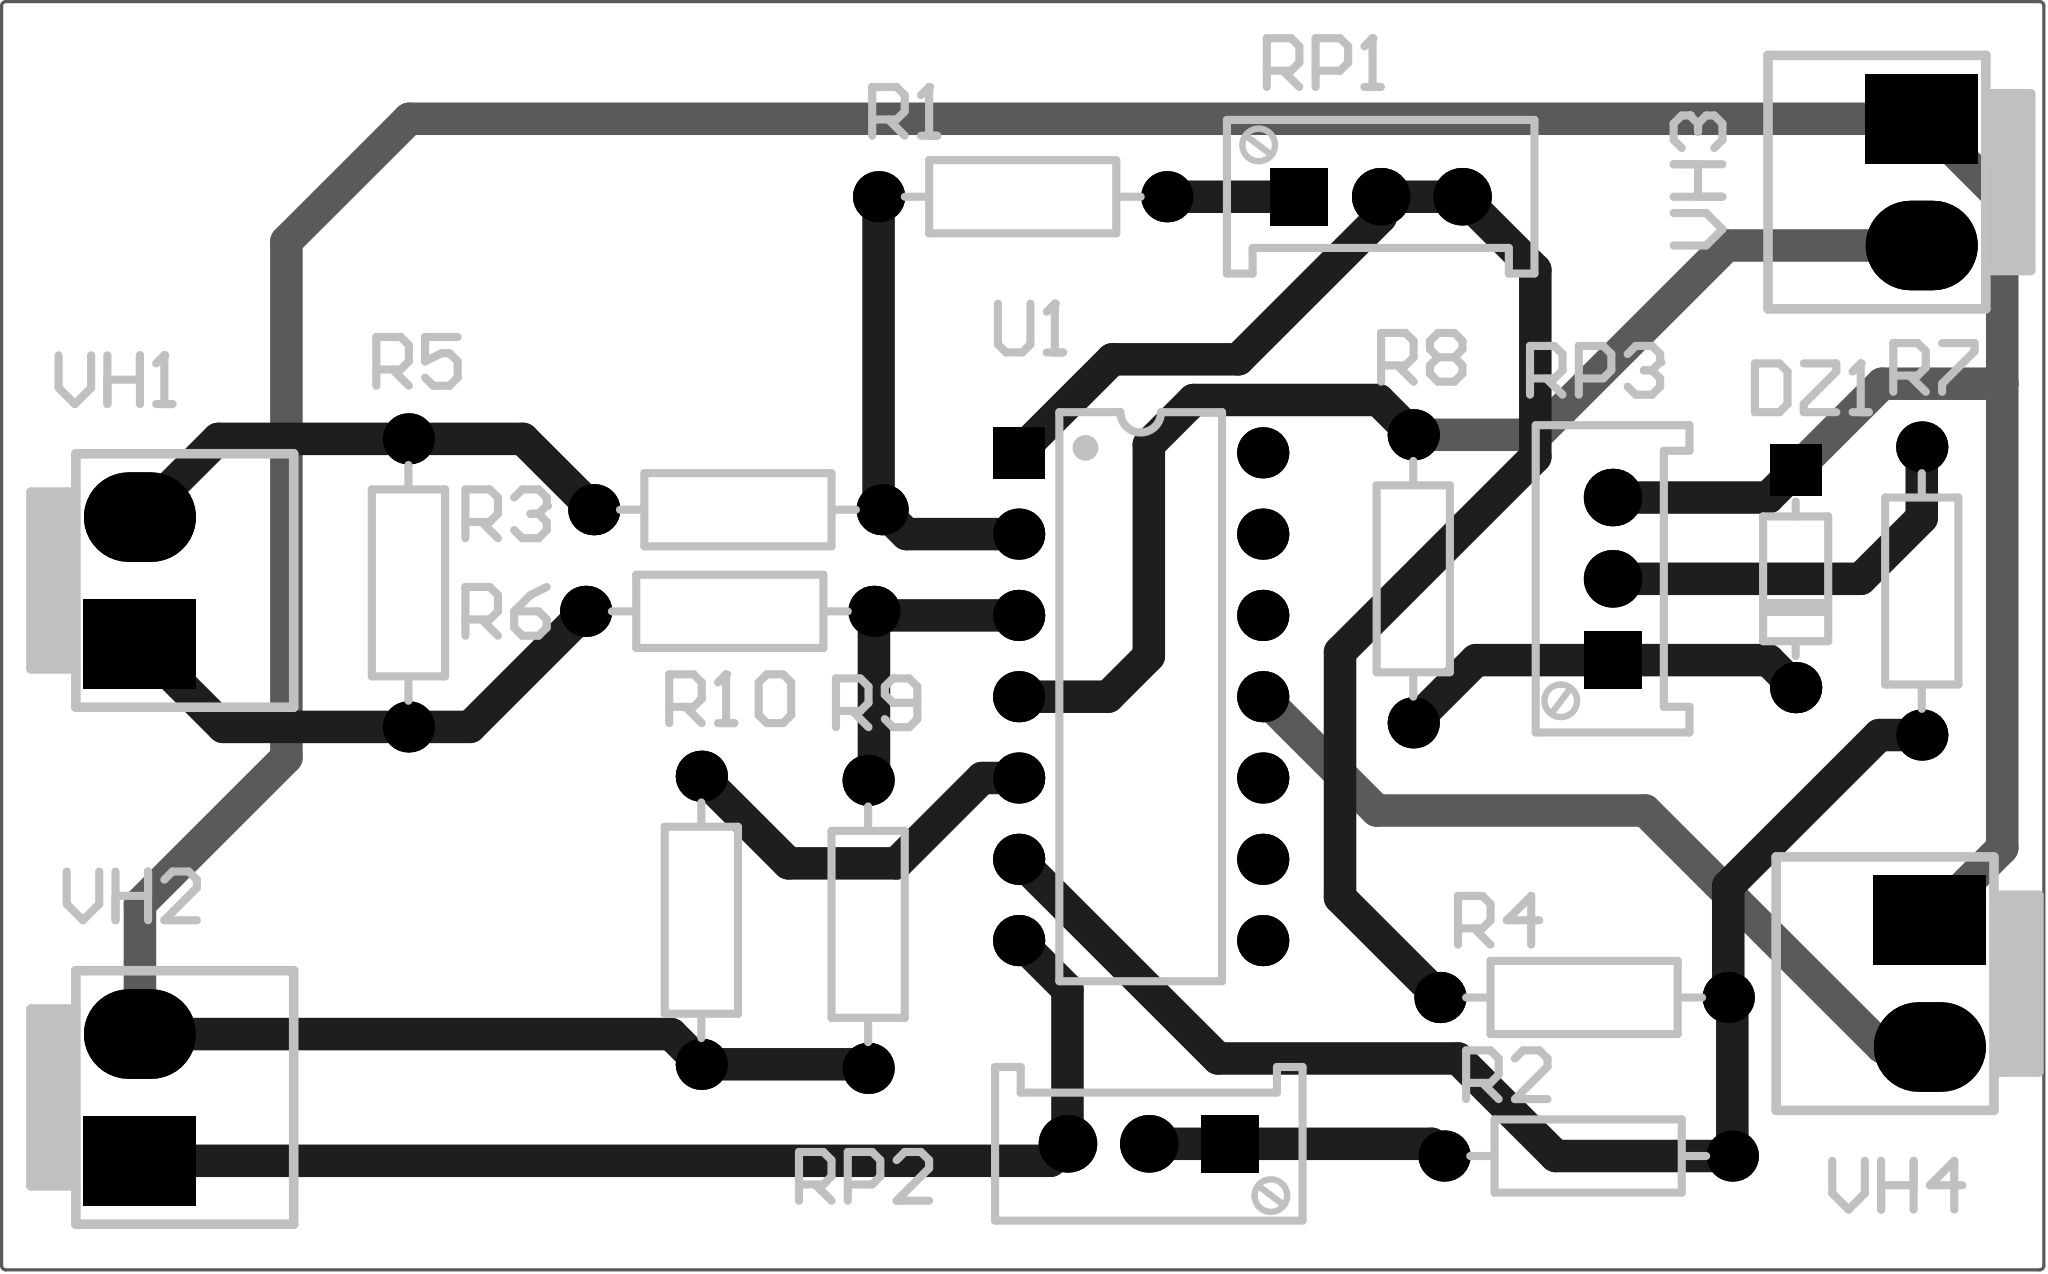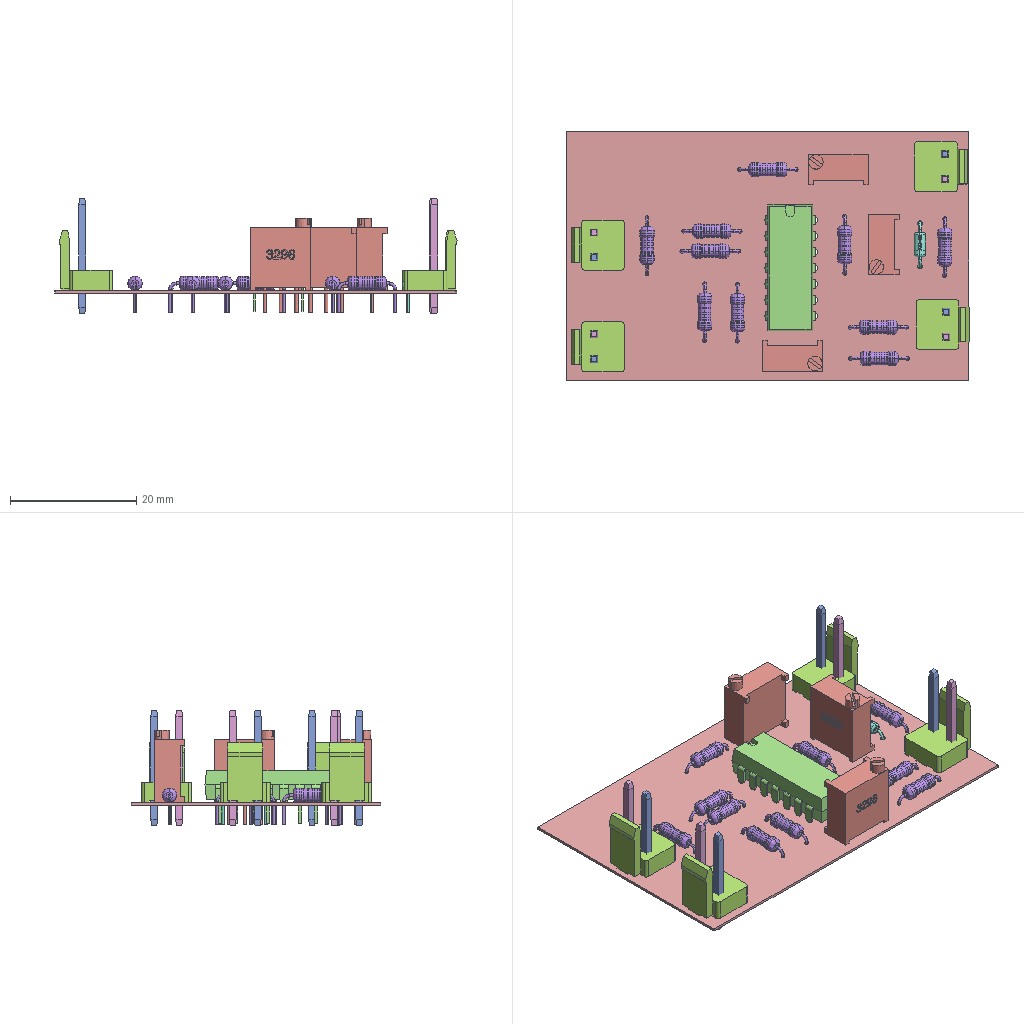Circuit board layout | Altium Designer | box 63.8 x 39.6 x 18.2 mm
Layer stack:
# Altium Designer layer stack of  (unit mm; dielectric type: 0 none, 1 core, 2 prepreg, 3 surface material)
index,name,kind,layer,copper_thickness_mm,dielectric_type,dielectric_thickness_mm,dielectric_material,dielectric_constant
0,Top Paste,other,,,,,,
1,Top Overlay,other,,,,,,
2,Top Solder,dielectric,,,3,0.0102,Solder Resist,3.5
3,Top Layer,copper,Top Layer,0.0356,,,,
4,Dielectric 1,dielectric,,,0,0.32,FR-4,4.8
5,Bottom Layer,copper,Bottom Layer,0.0356,,,,
6,Bottom Solder,dielectric,,,3,0.0102,Solder Resist,3.5
7,Bottom Overlay,other,,,,,,
8,Bottom Paste,other,,,,,,
# drill layer pairs: low layer,high layer
drill_pair,Top Layer,Bottom Layer
Part placement:
Designator,Comment,Layer,Footprint,Center-X(mm),Center-Y(mm),Rotation
VH4,VH2,TopLayer,VH3.96-2A,122.301,34.215,270
VH3,VH2,TopLayer,VH3.96-2A,122.047,59.257,270
DZ1,6V2,TopLayer,DO-35,118.11,46.863,270
R1,9.1K,TopLayer,RS_1/4W,93.98,58.801,360
R2,22K,TopLayer,RS_1/4W,111.633,28.829,180
R3,10K,TopLayer,RS_1/4W,85.09,49.022,360
R4,10K,TopLayer,RS_1/4W,111.506,33.782,360
R5,500,TopLayer,RS_1/4W,74.803,46.736,90
R6,10K,TopLayer,RS_1/4W,84.836,45.847,360
R7,10K,TopLayer,RS_1/4W,122.047,46.482,270
R8,750,TopLayer,RS_1/4W,106.172,46.863,90
R9,10K,TopLayer,RS_1/4W,89.154,36.068,90
R10,3.9K,TopLayer,RS_1/4W,83.947,36.195,90
RP1,2K,TopLayer,3296W,105.156,58.801,360
RP2,5K,TopLayer,3296W,97.917,29.21,180
RP3,2K,TopLayer,3296W,112.395,46.863,90
U1,LM124AD,TopLayer,DIP14,97.663,43.18,0
VH1,VH2,TopLayer,VH3.96-2A,66.421,46.811,90
VH2,VH2,TopLayer,VH3.96-2A,66.421,30.659,90
Pad and via stacks:
# Altium Designer via and pad stacks of  (unit mm). Each distinct definition once, with the count of objects using it.
# via: kind,start_layer,end_layer,hole_mm,diameter_mm,mode(0 simple;1 top-mid-bottom;2 full stack),diameter_per_layer,count,example_net
# pad: kind,layer,hole_mm,hole_type(0 round;1 square;2 slot),plating,top_size,top_shape(1 round;2 rect;3 octagon;9 rounded rect),mid_size,bottom_size,mode,footprint,size_per_layer,count,example
pad,Multi-Layer,1.6,0,plated,2.8x3.5,2,2.8x3.5,2.8x3.5,0,VH3.96-2A,,4,VH3.1
pad,Multi-Layer,1.6,0,plated,2.8x3.5,1,2.8x3.5,2.8x3.5,0,VH3.96-2A,,4,VH3.2
pad,Multi-Layer,0.8,0,plated,1.6x1.6,2,1.6x1.6,1.6x1.6,0,DO-35,,1,DZ1.1
pad,Multi-Layer,0.8,0,plated,1.6x1.6,1,1.6x1.6,1.6x1.6,0,DO-35,,1,DZ1.2
pad,Multi-Layer,0.7,0,plated,1.8x1.8,2,1.8x1.8,1.8x1.8,0,3296W,,3,RP3.1
pad,Multi-Layer,0.7,0,plated,1.8x1.8,1,1.8x1.8,1.8x1.8,0,3296W,,6,RP3.2
pad,Multi-Layer,0.6,0,plated,1.6x1.6,1,1.6x1.6,1.6x1.6,0,RS 1/4W,,20,R10.1
pad,Multi-Layer,0.8128,0,plated,1.6x1.6,2,1.6x1.6,1.6x1.6,0,DIP14,,1,U1.1
pad,Multi-Layer,0.8128,0,plated,1.6x1.6,1,1.6x1.6,1.6x1.6,0,DIP14,,13,U1.2
Design rules, without the lines most boards share:
# Altium Designer design rules of  (exported by Altium Designer, unit mm)
# columns: name | kind | enabled | priority | scope1 | scope2 | descriptor | typed fields (field=value)
Clearance | 0 | enabled | 1 | All | All | Clearance Constraint (Gap=10mil) (All),(All) | gap=0.254
PlaneConnect | 6 | enabled | 1 | All | All | Power Plane Connect Rule(Relief Connect )(Expansion=20mil) (Conductor Width=10mil) (Air Gap=10mil) (Entries=4) (All) | relief_conductor_width=0.254 relief_entries=4 relief_expansion=0.508
PolygonConnect | 20 | enabled | 1 | All | All | Polygon Connect Rule(Relief Connect )(Conductor Width=10mil) (Relief Angle=90 Angle) (Entries=4) (Air Gap Width=10mil) (All),(All) | connect_style(0=relief,1=direct,2=none)=0 relief_conductor_width=0.254 relief_entries=4
Width | 2 | enabled | 1 | All | All | Width Constraint (Min=40mil) (Max=40mil) (Preferred=40mil) (All) |
RoutingVias | 11 | enabled | 1 | All | All | Routing Via (MinHoleWidth=28mil) (MaxHoleWidth=28mil) (PreferredHoleWidth=28mil) (MinWidth=50mil) (MaxWidth=50mil) (PreferedWidth=50mil) (All) | via_min_hole=0.7112 via_max_hole=0.7112 via_preferred_diameter=1.27 via_preferred_hole=0.7112
PasteMaskExpansion | 14 | enabled | 1 | All | All | Paste Mask Expansion (Expansion =0mil) (All) | expansion=0
SolderMaskExpansion | 13 | enabled | 1 | All | All | Solder Mask Expansion (Expansion =4mil) (All) | expansion=0.1016
DiffPairsRouting | 51 | enabled | 1 | All | All | Differential Pairs Uncoupled Length using the Gap Constraints (Min=10mil) (Max=10mil) (Prefered=10mil)  and Width Constraints (Min=15mil) (Max=15mil) (Prefered=15mil) (All) |
HoleToHoleClearance | 52 | enabled | 1 | All | All | Hole To Hole Clearance (Gap=10mil) (All),(All) | gap=0.254
MinimumSolderMaskSliver | 53 | enabled | 1 | All | All | Minimum Solder Mask Sliver (Gap=0mil) (All),(All) |
SilkToSolderMaskClearance | 54 | enabled | 1 | IsPad | All | Silk To Solder Mask (Clearance=0mil) (IsPad),(All) |
SilkToSilkClearance | 55 | enabled | 1 | All | All | Silk to Silk (Clearance=0mil) (All),(All) |
Classes set for this board:
# Altium Designer classes of  (member kind: 0 net, 1 component, 2 from-to, 3 pad, 4 layer, 5 differential pair, 6 design channel, 7 polygon, 8 structure, 9 xSignal)
# columns: class name | member kind | superclass | members
Sheet1 | 1 | no | DZ1; R1; R2; R3; R4; R5; R6; R7; R8; R9; R10; RP1; RP2; RP3; U1; VH1; VH2; VH3; VH4;